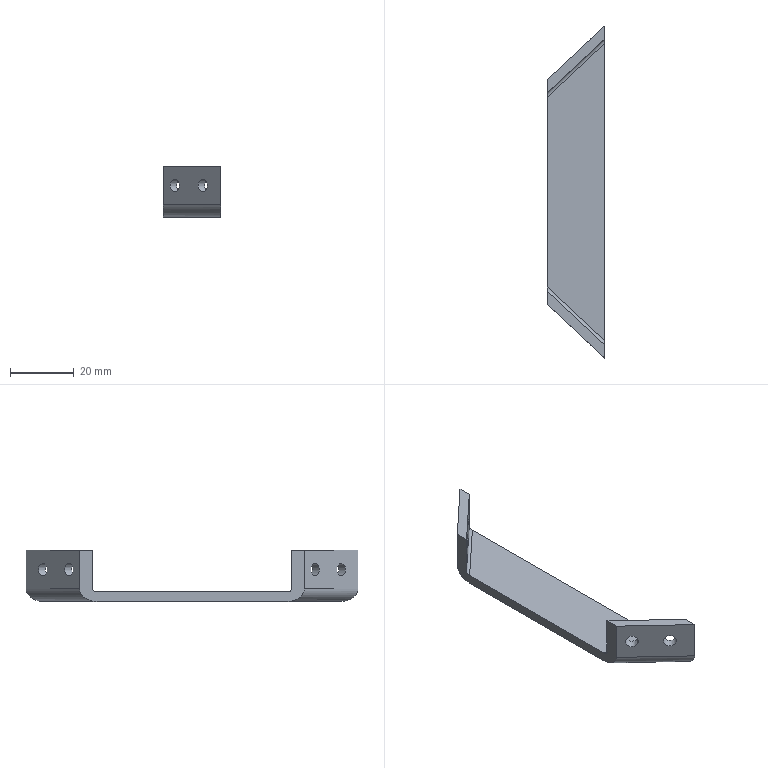Part | STEP file | 1-53.7 | 1 solid | 18 faces | box 18 x 104.1 x 16 mm | volume 6325 mm3 | plane 10 | cylinder 8 | commonest cylinder face diameters 4 x4 2 x2 8 x2